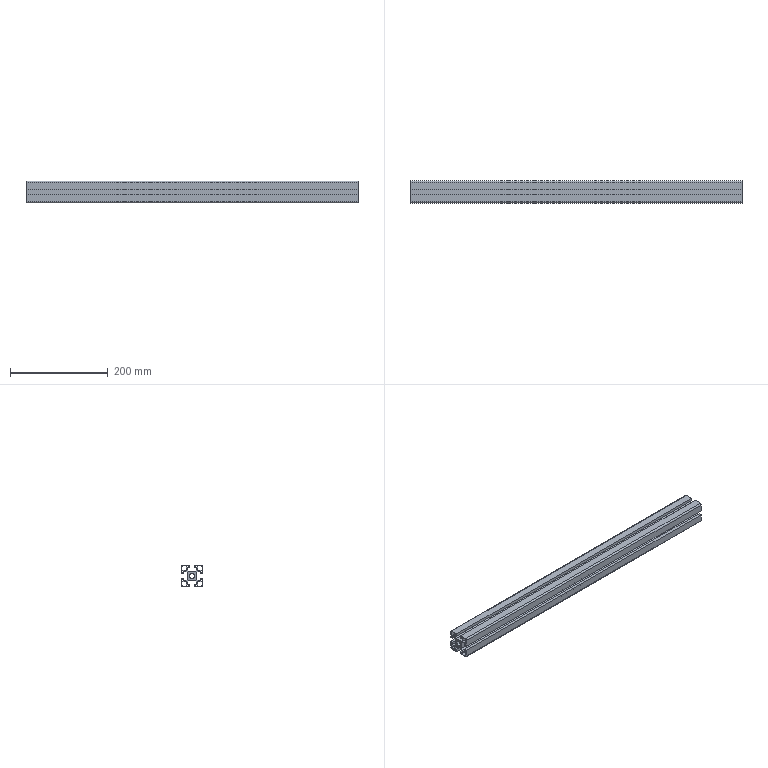Part | STEP file | 1_4 | 1 solid | 87 faces | box 680 x 45 x 45 mm | volume 556065 mm3 | plane 78 | cylinder 9 | commonest cylinder face diameters 2 x4 6 x4 10 x1